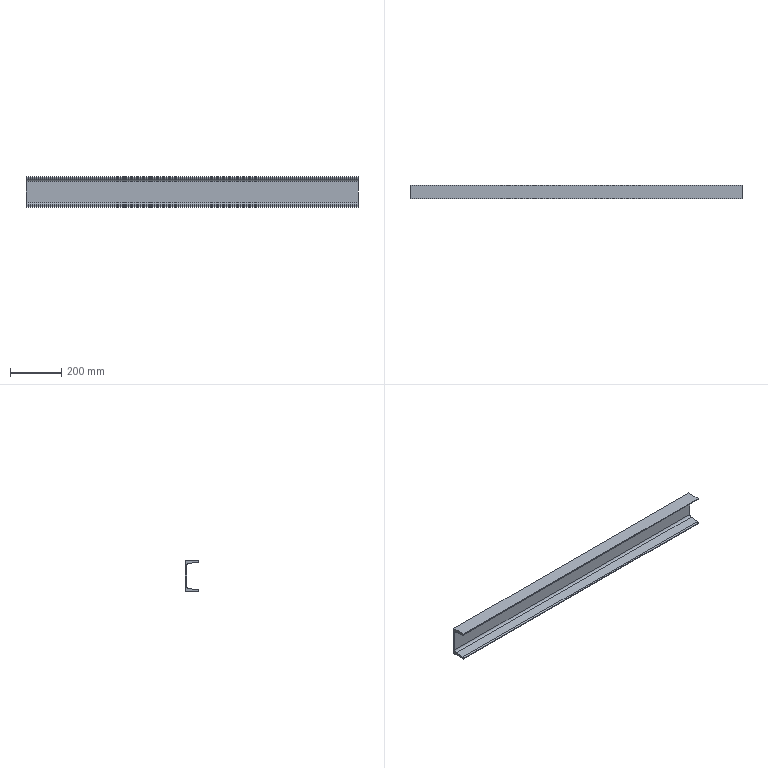Part | SolidWorks | features WeldMemberFeat 1, WeldmentFeature 1 | 1 solid | 14 faces | box 1300 x 53 x 120 mm | volume 1996260 mm3 | plane 10 | cylinder 4 | commonest cylinder face diameters 9 x2 18 x2
STEP:
#1=CARTESIAN_POINT('',(-650.,-53.,-120.));
#2=VERTEX_POINT('',#1);
#3=CARTESIAN_POINT('',(-650.,0.,-120.));
#4=VERTEX_POINT('',#3);
#5=CARTESIAN_POINT('',(-650.,0.,-120.));
#6=DIRECTION('',(0.,1.,0.));
#7=VECTOR('',#6,1000.);
#8=LINE('',#5,#7);
#9=EDGE_CURVE('',#2,#4,#8,.T.);
#10=ORIENTED_EDGE('',*,*,#9,.T.);
#11=CARTESIAN_POINT('',(650.,0.,-120.));
#12=VERTEX_POINT('',#11);
#13=CARTESIAN_POINT('',(650.,0.,-120.));
#14=DIRECTION('',(-1.,0.,0.));
#15=VECTOR('',#14,1000.);
#16=LINE('',#13,#15);
#17=EDGE_CURVE('',#12,#4,#16,.T.);
#18=ORIENTED_EDGE('',*,*,#17,.F.);
#19=CARTESIAN_POINT('',(650.,-53.,-120.));
#20=VERTEX_POINT('',#19);
#21=CARTESIAN_POINT('',(650.,0.,-120.));
#22=DIRECTION('',(0.,1.,0.));
#23=VECTOR('',#22,1000.);
#24=LINE('',#21,#23);
#25=EDGE_CURVE('',#20,#12,#24,.T.);
#26=ORIENTED_EDGE('',*,*,#25,.F.);
#27=CARTESIAN_POINT('',(650.,-53.,-120.));
#28=DIRECTION('',(-1.,0.,0.));
#29=VECTOR('',#28,1000.);
#30=LINE('',#27,#29);
#31=EDGE_CURVE('',#20,#2,#30,.T.);
#32=ORIENTED_EDGE('',*,*,#31,.T.);
#33=EDGE_LOOP('',(#10,#18,#26,#32));
#34=FACE_OUTER_BOUND('',#33,.T.);
#35=CARTESIAN_POINT('',(650.,0.,-120.));
#36=DIRECTION('',(0.,0.,1.));
#37=DIRECTION('',(1.,0.,0.));
#38=AXIS2_PLACEMENT_3D('',#35,#36,#37);
#39=PLANE('',#38);
#40=ADVANCED_FACE('',(#34),#39,.F.);
#41=CARTESIAN_POINT('',(-650.,0.,0.));
#42=VERTEX_POINT('',#41);
#43=CARTESIAN_POINT('',(-650.,0.,0.));
#44=DIRECTION('',(0.,0.,1.));
#45=VECTOR('',#44,1000.);
#46=LINE('',#43,#45);
#47=EDGE_CURVE('',#4,#42,#46,.T.);
#48=ORIENTED_EDGE('',*,*,#47,.T.);
#49=CARTESIAN_POINT('',(650.,0.,0.));
#50=VERTEX_POINT('',#49);
#51=CARTESIAN_POINT('',(650.,0.,0.));
#52=DIRECTION('',(-1.,0.,0.));
#53=VECTOR('',#52,1000.);
#54=LINE('',#51,#53);
#55=EDGE_CURVE('',#50,#42,#54,.T.);
#56=ORIENTED_EDGE('',*,*,#55,.F.);
#57=CARTESIAN_POINT('',(650.,0.,0.));
#58=DIRECTION('',(0.,0.,1.));
#59=VECTOR('',#58,1000.);
#60=LINE('',#57,#59);
#61=EDGE_CURVE('',#12,#50,#60,.T.);
#62=ORIENTED_EDGE('',*,*,#61,.F.);
#63=ORIENTED_EDGE('',*,*,#17,.T.);
#64=EDGE_LOOP('',(#48,#56,#62,#63));
#65=FACE_OUTER_BOUND('',#64,.T.);
#66=CARTESIAN_POINT('',(650.,0.,0.));
#67=DIRECTION('',(0.,-1.,0.));
#68=DIRECTION('',(1.,0.,0.));
#69=AXIS2_PLACEMENT_3D('',#66,#67,#68);
#70=PLANE('',#69);
#71=ADVANCED_FACE('',(#65),#70,.F.);
#72=CARTESIAN_POINT('',(-650.,-53.,0.));
#73=VERTEX_POINT('',#72);
#74=CARTESIAN_POINT('',(-650.,0.,0.));
#75=DIRECTION('',(0.,-1.,0.));
#76=VECTOR('',#75,1000.);
#77=LINE('',#74,#76);
#78=EDGE_CURVE('',#42,#73,#77,.T.);
#79=ORIENTED_EDGE('',*,*,#78,.T.);
#80=CARTESIAN_POINT('',(650.,-53.,0.));
#81=VERTEX_POINT('',#80);
#82=CARTESIAN_POINT('',(650.,-53.,0.));
#83=DIRECTION('',(-1.,0.,0.));
#84=VECTOR('',#83,1000.);
#85=LINE('',#82,#84);
#86=EDGE_CURVE('',#81,#73,#85,.T.);
#87=ORIENTED_EDGE('',*,*,#86,.F.);
#88=CARTESIAN_POINT('',(650.,0.,0.));
#89=DIRECTION('',(0.,-1.,0.));
#90=VECTOR('',#89,1000.);
#91=LINE('',#88,#90);
#92=EDGE_CURVE('',#50,#81,#91,.T.);
#93=ORIENTED_EDGE('',*,*,#92,.F.);
#94=ORIENTED_EDGE('',*,*,#55,.T.);
#95=EDGE_LOOP('',(#79,#87,#93,#94));
#96=FACE_OUTER_BOUND('',#95,.T.);
#97=CARTESIAN_POINT('',(650.,0.,0.));
#98=DIRECTION('',(0.,0.,-1.));
#99=DIRECTION('',(0.,1.,0.));
#100=AXIS2_PLACEMENT_3D('',#97,#98,#99);
#101=PLANE('',#100);
#102=ADVANCED_FACE('',(#96),#101,.F.);
#103=CARTESIAN_POINT('',(-650.,-53.,-2.553));
#104=VERTEX_POINT('',#103);
#105=CARTESIAN_POINT('',(-650.,-53.,-2.553));
#106=DIRECTION('',(0.,0.,-1.));
#107=VECTOR('',#106,1000.);
#108=LINE('',#105,#107);
#109=EDGE_CURVE('',#73,#104,#108,.T.);
#110=ORIENTED_EDGE('',*,*,#109,.T.);
#111=CARTESIAN_POINT('',(650.,-53.,-2.553));
#112=VERTEX_POINT('',#111);
#113=CARTESIAN_POINT('',(650.,-53.,-2.553));
#114=DIRECTION('',(-1.,0.,0.));
#115=VECTOR('',#114,1000.);
#116=LINE('',#113,#115);
#117=EDGE_CURVE('',#112,#104,#116,.T.);
#118=ORIENTED_EDGE('',*,*,#117,.F.);
#119=CARTESIAN_POINT('',(650.,-53.,-2.553));
#120=DIRECTION('',(0.,0.,-1.));
#121=VECTOR('',#120,1000.);
#122=LINE('',#119,#121);
#123=EDGE_CURVE('',#81,#112,#122,.T.);
#124=ORIENTED_EDGE('',*,*,#123,.F.);
#125=ORIENTED_EDGE('',*,*,#86,.T.);
#126=EDGE_LOOP('',(#110,#118,#124,#125));
#127=FACE_OUTER_BOUND('',#126,.T.);
#128=CARTESIAN_POINT('',(650.,-53.,-2.553));
#129=DIRECTION('',(0.,1.,0.));
#130=DIRECTION('',(0.,0.,1.));
#131=AXIS2_PLACEMENT_3D('',#128,#129,#130);
#132=PLANE('',#131);
#133=ADVANCED_FACE('',(#127),#132,.F.);
#134=CARTESIAN_POINT('',(-650.,-48.948,-7.03));
#135=VERTEX_POINT('',#134);
#136=CARTESIAN_POINT('',(-650.,-48.5,-2.553));
#137=DIRECTION('',(1.,0.,0.));
#138=DIRECTION('',(0.,1.,0.));
#139=AXIS2_PLACEMENT_3D('',#136,#137,#138);
#140=CIRCLE('',#139,4.5);
#141=EDGE_CURVE('',#104,#135,#140,.T.);
#142=ORIENTED_EDGE('',*,*,#141,.T.);
#143=CARTESIAN_POINT('',(650.,-48.948,-7.03));
#144=VERTEX_POINT('',#143);
#145=CARTESIAN_POINT('',(650.,-48.948,-7.03));
#146=DIRECTION('',(-1.,0.,0.));
#147=VECTOR('',#146,1000.);
#148=LINE('',#145,#147);
#149=EDGE_CURVE('',#144,#135,#148,.T.);
#150=ORIENTED_EDGE('',*,*,#149,.F.);
#151=CARTESIAN_POINT('',(650.,-48.5,-2.553));
#152=DIRECTION('',(1.,0.,0.));
#153=DIRECTION('',(0.,1.,0.));
#154=AXIS2_PLACEMENT_3D('',#151,#152,#153);
#155=CIRCLE('',#154,4.5);
#156=EDGE_CURVE('',#112,#144,#155,.T.);
#157=ORIENTED_EDGE('',*,*,#156,.F.);
#158=ORIENTED_EDGE('',*,*,#117,.T.);
#159=EDGE_LOOP('',(#142,#150,#157,#158));
#160=FACE_OUTER_BOUND('',#159,.T.);
#161=CARTESIAN_POINT('',(650.,-48.5,-2.553));
#162=DIRECTION('',(-1.,0.,0.));
#163=DIRECTION('',(0.,-1.,0.));
#164=AXIS2_PLACEMENT_3D('',#161,#162,#163);
#165=CYLINDRICAL_SURFACE('',#164,4.5);
#166=ADVANCED_FACE('',(#160),#165,.T.);
#167=CARTESIAN_POINT('',(-650.,-13.604,-10.565));
#168=VERTEX_POINT('',#167);
#169=CARTESIAN_POINT('',(-650.,-13.604,-10.565));
#170=DIRECTION('',(0.,0.995,-0.0995));
#171=VECTOR('',#170,1000.);
#172=LINE('',#169,#171);
#173=EDGE_CURVE('',#135,#168,#172,.T.);
#174=ORIENTED_EDGE('',*,*,#173,.T.);
#175=CARTESIAN_POINT('',(650.,-13.604,-10.565));
#176=VERTEX_POINT('',#175);
#177=CARTESIAN_POINT('',(650.,-13.604,-10.565));
#178=DIRECTION('',(-1.,0.,0.));
#179=VECTOR('',#178,1000.);
#180=LINE('',#177,#179);
#181=EDGE_CURVE('',#176,#168,#180,.T.);
#182=ORIENTED_EDGE('',*,*,#181,.F.);
#183=CARTESIAN_POINT('',(650.,-13.604,-10.565));
#184=DIRECTION('',(0.,0.995,-0.0995));
#185=VECTOR('',#184,1000.);
#186=LINE('',#183,#185);
#187=EDGE_CURVE('',#144,#176,#186,.T.);
#188=ORIENTED_EDGE('',*,*,#187,.F.);
#189=ORIENTED_EDGE('',*,*,#149,.T.);
#190=EDGE_LOOP('',(#174,#182,#188,#189));
#191=FACE_OUTER_BOUND('',#190,.T.);
#192=CARTESIAN_POINT('',(650.,-13.604,-10.565));
#193=DIRECTION('',(0.,0.0995,0.995));
#194=DIRECTION('',(0.,-0.995,0.0995));
#195=AXIS2_PLACEMENT_3D('',#192,#193,#194);
#196=PLANE('',#195);
#197=ADVANCED_FACE('',(#191),#196,.F.);
#198=CARTESIAN_POINT('',(-650.,-5.5,-19.52));
#199=VERTEX_POINT('',#198);
#200=CARTESIAN_POINT('',(-650.,-14.5,-19.52));
#201=DIRECTION('',(-1.,0.,0.));
#202=DIRECTION('',(0.,-1.,0.));
#203=AXIS2_PLACEMENT_3D('',#200,#201,#202);
#204=CIRCLE('',#203,9.);
#205=EDGE_CURVE('',#168,#199,#204,.T.);
#206=ORIENTED_EDGE('',*,*,#205,.T.);
#207=CARTESIAN_POINT('',(650.,-5.5,-19.52));
#208=VERTEX_POINT('',#207);
#209=CARTESIAN_POINT('',(650.,-5.5,-19.52));
#210=DIRECTION('',(-1.,0.,0.));
#211=VECTOR('',#210,1000.);
#212=LINE('',#209,#211);
#213=EDGE_CURVE('',#208,#199,#212,.T.);
#214=ORIENTED_EDGE('',*,*,#213,.F.);
#215=CARTESIAN_POINT('',(650.,-14.5,-19.52));
#216=DIRECTION('',(-1.,0.,0.));
#217=DIRECTION('',(0.,-1.,0.));
#218=AXIS2_PLACEMENT_3D('',#215,#216,#217);
#219=CIRCLE('',#218,9.);
#220=EDGE_CURVE('',#176,#208,#219,.T.);
#221=ORIENTED_EDGE('',*,*,#220,.F.);
#222=ORIENTED_EDGE('',*,*,#181,.T.);
#223=EDGE_LOOP('',(#206,#214,#221,#222));
#224=FACE_OUTER_BOUND('',#223,.T.);
#225=CARTESIAN_POINT('',(650.,-14.5,-19.52));
#226=DIRECTION('',(-1.,0.,0.));
#227=DIRECTION('',(0.,-1.,0.));
#228=AXIS2_PLACEMENT_3D('',#225,#226,#227);
#229=CYLINDRICAL_SURFACE('',#228,9.);
#230=ADVANCED_FACE('',(#224),#229,.F.);
#231=CARTESIAN_POINT('',(-650.,-5.5,-100.48));
#232=VERTEX_POINT('',#231);
#233=CARTESIAN_POINT('',(-650.,-5.5,-100.48));
#234=DIRECTION('',(0.,0.,-1.));
#235=VECTOR('',#234,1000.);
#236=LINE('',#233,#235);
#237=EDGE_CURVE('',#199,#232,#236,.T.);
#238=ORIENTED_EDGE('',*,*,#237,.T.);
#239=CARTESIAN_POINT('',(650.,-5.5,-100.48));
#240=VERTEX_POINT('',#239);
#241=CARTESIAN_POINT('',(650.,-5.5,-100.48));
#242=DIRECTION('',(-1.,0.,0.));
#243=VECTOR('',#242,1000.);
#244=LINE('',#241,#243);
#245=EDGE_CURVE('',#240,#232,#244,.T.);
#246=ORIENTED_EDGE('',*,*,#245,.F.);
#247=CARTESIAN_POINT('',(650.,-5.5,-100.48));
#248=DIRECTION('',(0.,0.,-1.));
#249=VECTOR('',#248,1000.);
#250=LINE('',#247,#249);
#251=EDGE_CURVE('',#208,#240,#250,.T.);
#252=ORIENTED_EDGE('',*,*,#251,.F.);
#253=ORIENTED_EDGE('',*,*,#213,.T.);
#254=EDGE_LOOP('',(#238,#246,#252,#253));
#255=FACE_OUTER_BOUND('',#254,.T.);
#256=CARTESIAN_POINT('',(650.,-5.5,-100.48));
#257=DIRECTION('',(0.,1.,0.));
#258=DIRECTION('',(0.,0.,1.));
#259=AXIS2_PLACEMENT_3D('',#256,#257,#258);
#260=PLANE('',#259);
#261=ADVANCED_FACE('',(#255),#260,.F.);
#262=CARTESIAN_POINT('',(-650.,-13.604,-109.435));
#263=VERTEX_POINT('',#262);
#264=CARTESIAN_POINT('',(-650.,-14.5,-100.48));
#265=DIRECTION('',(-1.,0.,0.));
#266=DIRECTION('',(0.,-1.,0.));
#267=AXIS2_PLACEMENT_3D('',#264,#265,#266);
#268=CIRCLE('',#267,9.);
#269=EDGE_CURVE('',#232,#263,#268,.T.);
#270=ORIENTED_EDGE('',*,*,#269,.T.);
#271=CARTESIAN_POINT('',(650.,-13.604,-109.435));
#272=VERTEX_POINT('',#271);
#273=CARTESIAN_POINT('',(650.,-13.604,-109.435));
#274=DIRECTION('',(-1.,0.,0.));
#275=VECTOR('',#274,1000.);
#276=LINE('',#273,#275);
#277=EDGE_CURVE('',#272,#263,#276,.T.);
#278=ORIENTED_EDGE('',*,*,#277,.F.);
#279=CARTESIAN_POINT('',(650.,-14.5,-100.48));
#280=DIRECTION('',(-1.,0.,0.));
#281=DIRECTION('',(0.,-1.,0.));
#282=AXIS2_PLACEMENT_3D('',#279,#280,#281);
#283=CIRCLE('',#282,9.);
#284=EDGE_CURVE('',#240,#272,#283,.T.);
#285=ORIENTED_EDGE('',*,*,#284,.F.);
#286=ORIENTED_EDGE('',*,*,#245,.T.);
#287=EDGE_LOOP('',(#270,#278,#285,#286));
#288=FACE_OUTER_BOUND('',#287,.T.);
#289=CARTESIAN_POINT('',(650.,-14.5,-100.48));
#290=DIRECTION('',(-1.,0.,0.));
#291=DIRECTION('',(0.,-1.,0.));
#292=AXIS2_PLACEMENT_3D('',#289,#290,#291);
#293=CYLINDRICAL_SURFACE('',#292,9.);
#294=ADVANCED_FACE('',(#288),#293,.F.);
#295=CARTESIAN_POINT('',(-650.,-48.948,-112.97));
#296=VERTEX_POINT('',#295);
#297=CARTESIAN_POINT('',(-650.,-13.604,-109.435));
#298=DIRECTION('',(0.,-0.995,-0.0995));
#299=VECTOR('',#298,1000.);
#300=LINE('',#297,#299);
#301=EDGE_CURVE('',#263,#296,#300,.T.);
#302=ORIENTED_EDGE('',*,*,#301,.T.);
#303=CARTESIAN_POINT('',(650.,-48.948,-112.97));
#304=VERTEX_POINT('',#303);
#305=CARTESIAN_POINT('',(650.,-48.948,-112.97));
#306=DIRECTION('',(-1.,0.,0.));
#307=VECTOR('',#306,1000.);
#308=LINE('',#305,#307);
#309=EDGE_CURVE('',#304,#296,#308,.T.);
#310=ORIENTED_EDGE('',*,*,#309,.F.);
#311=CARTESIAN_POINT('',(650.,-13.604,-109.435));
#312=DIRECTION('',(0.,-0.995,-0.0995));
#313=VECTOR('',#312,1000.);
#314=LINE('',#311,#313);
#315=EDGE_CURVE('',#272,#304,#314,.T.);
#316=ORIENTED_EDGE('',*,*,#315,.F.);
#317=ORIENTED_EDGE('',*,*,#277,.T.);
#318=EDGE_LOOP('',(#302,#310,#316,#317));
#319=FACE_OUTER_BOUND('',#318,.T.);
#320=CARTESIAN_POINT('',(650.,-13.604,-109.435));
#321=DIRECTION('',(0.,0.0995,-0.995));
#322=DIRECTION('',(0.,0.995,0.0995));
#323=AXIS2_PLACEMENT_3D('',#320,#321,#322);
#324=PLANE('',#323);
#325=ADVANCED_FACE('',(#319),#324,.F.);
#326=CARTESIAN_POINT('',(-650.,-53.,-117.447));
#327=VERTEX_POINT('',#326);
#328=CARTESIAN_POINT('',(-650.,-48.5,-117.447));
#329=DIRECTION('',(1.,0.,0.));
#330=DIRECTION('',(0.,1.,0.));
#331=AXIS2_PLACEMENT_3D('',#328,#329,#330);
#332=CIRCLE('',#331,4.5);
#333=EDGE_CURVE('',#296,#327,#332,.T.);
#334=ORIENTED_EDGE('',*,*,#333,.T.);
#335=CARTESIAN_POINT('',(650.,-53.,-117.447));
#336=VERTEX_POINT('',#335);
#337=CARTESIAN_POINT('',(650.,-53.,-117.447));
#338=DIRECTION('',(-1.,0.,0.));
#339=VECTOR('',#338,1000.);
#340=LINE('',#337,#339);
#341=EDGE_CURVE('',#336,#327,#340,.T.);
#342=ORIENTED_EDGE('',*,*,#341,.F.);
#343=CARTESIAN_POINT('',(650.,-48.5,-117.447));
#344=DIRECTION('',(1.,0.,0.));
#345=DIRECTION('',(0.,1.,0.));
#346=AXIS2_PLACEMENT_3D('',#343,#344,#345);
#347=CIRCLE('',#346,4.5);
#348=EDGE_CURVE('',#304,#336,#347,.T.);
#349=ORIENTED_EDGE('',*,*,#348,.F.);
#350=ORIENTED_EDGE('',*,*,#309,.T.);
#351=EDGE_LOOP('',(#334,#342,#349,#350));
#352=FACE_OUTER_BOUND('',#351,.T.);
#353=CARTESIAN_POINT('',(650.,-48.5,-117.447));
#354=DIRECTION('',(-1.,0.,0.));
#355=DIRECTION('',(0.,-1.,0.));
#356=AXIS2_PLACEMENT_3D('',#353,#354,#355);
#357=CYLINDRICAL_SURFACE('',#356,4.5);
#358=ADVANCED_FACE('',(#352),#357,.T.);
#359=CARTESIAN_POINT('',(-650.,-53.,-117.447));
#360=DIRECTION('',(0.,0.,-1.));
#361=VECTOR('',#360,1000.);
#362=LINE('',#359,#361);
#363=EDGE_CURVE('',#327,#2,#362,.T.);
#364=ORIENTED_EDGE('',*,*,#363,.T.);
#365=ORIENTED_EDGE('',*,*,#31,.F.);
#366=CARTESIAN_POINT('',(650.,-53.,-117.447));
#367=DIRECTION('',(0.,0.,-1.));
#368=VECTOR('',#367,1000.);
#369=LINE('',#366,#368);
#370=EDGE_CURVE('',#336,#20,#369,.T.);
#371=ORIENTED_EDGE('',*,*,#370,.F.);
#372=ORIENTED_EDGE('',*,*,#341,.T.);
#373=EDGE_LOOP('',(#364,#365,#371,#372));
#374=FACE_OUTER_BOUND('',#373,.T.);
#375=CARTESIAN_POINT('',(650.,-53.,-117.447));
#376=DIRECTION('',(0.,1.,0.));
#377=DIRECTION('',(0.,0.,1.));
#378=AXIS2_PLACEMENT_3D('',#375,#376,#377);
#379=PLANE('',#378);
#380=ADVANCED_FACE('',(#374),#379,.F.);
#381=ORIENTED_EDGE('',*,*,#25,.T.);
#382=ORIENTED_EDGE('',*,*,#61,.T.);
#383=ORIENTED_EDGE('',*,*,#92,.T.);
#384=ORIENTED_EDGE('',*,*,#123,.T.);
#385=ORIENTED_EDGE('',*,*,#156,.T.);
#386=ORIENTED_EDGE('',*,*,#187,.T.);
#387=ORIENTED_EDGE('',*,*,#220,.T.);
#388=ORIENTED_EDGE('',*,*,#251,.T.);
#389=ORIENTED_EDGE('',*,*,#284,.T.);
#390=ORIENTED_EDGE('',*,*,#315,.T.);
#391=ORIENTED_EDGE('',*,*,#348,.T.);
#392=ORIENTED_EDGE('',*,*,#370,.T.);
#393=EDGE_LOOP('',(#381,#382,#383,#384,#385,#386,#387,#388,#389,#390,#391,#392));
#394=FACE_OUTER_BOUND('',#393,.T.);
#395=CARTESIAN_POINT('',(650.,-48.5,-117.447));
#396=DIRECTION('',(1.,0.,0.));
#397=DIRECTION('',(0.,1.,0.));
#398=AXIS2_PLACEMENT_3D('',#395,#396,#397);
#399=PLANE('',#398);
#400=ADVANCED_FACE('',(#394),#399,.T.);
#401=ORIENTED_EDGE('',*,*,#9,.F.);
#402=ORIENTED_EDGE('',*,*,#363,.F.);
#403=ORIENTED_EDGE('',*,*,#333,.F.);
#404=ORIENTED_EDGE('',*,*,#301,.F.);
#405=ORIENTED_EDGE('',*,*,#269,.F.);
#406=ORIENTED_EDGE('',*,*,#237,.F.);
#407=ORIENTED_EDGE('',*,*,#205,.F.);
#408=ORIENTED_EDGE('',*,*,#173,.F.);
#409=ORIENTED_EDGE('',*,*,#141,.F.);
#410=ORIENTED_EDGE('',*,*,#109,.F.);
#411=ORIENTED_EDGE('',*,*,#78,.F.);
#412=ORIENTED_EDGE('',*,*,#47,.F.);
#413=EDGE_LOOP('',(#401,#402,#403,#404,#405,#406,#407,#408,#409,#410,#411,#412));
#414=FACE_OUTER_BOUND('',#413,.T.);
#415=CARTESIAN_POINT('',(-650.,-48.5,-117.447));
#416=DIRECTION('',(1.,0.,0.));
#417=DIRECTION('',(0.,1.,0.));
#418=AXIS2_PLACEMENT_3D('',#415,#416,#417);
#419=PLANE('',#418);
#420=ADVANCED_FACE('',(#414),#419,.F.);
#421=CLOSED_SHELL('',(#40,#71,#102,#133,#166,#197,#230,#261,#294,#325,#358,#380,#400,#420));
#422=MANIFOLD_SOLID_BREP('',#421);
#423=CARTESIAN_POINT('',(0.,0.,0.));
#424=DIRECTION('',(0.,0.,1.));
#425=DIRECTION('',(1.,0.,0.));
#426=AXIS2_PLACEMENT_3D('',#423,#424,#425);
#427=(LENGTH_UNIT()NAMED_UNIT(*)SI_UNIT(.MILLI.,.METRE.));
#428=UNCERTAINTY_MEASURE_WITH_UNIT(LENGTH_MEASURE(0.00001),#427,'','');
#429=(NAMED_UNIT(*)PLANE_ANGLE_UNIT()SI_UNIT($,.RADIAN.));
#430=(NAMED_UNIT(*)SI_UNIT($,.STERADIAN.)SOLID_ANGLE_UNIT());
#431=(GEOMETRIC_REPRESENTATION_CONTEXT(3)GLOBAL_UNCERTAINTY_ASSIGNED_CONTEXT((#428))GLOBAL_UNIT_ASSIGNED_CONTEXT((#427,#429,#430))REPRESENTATION_CONTEXT('',''));
#432=ADVANCED_BREP_SHAPE_REPRESENTATION('',(#422,#426),#431);